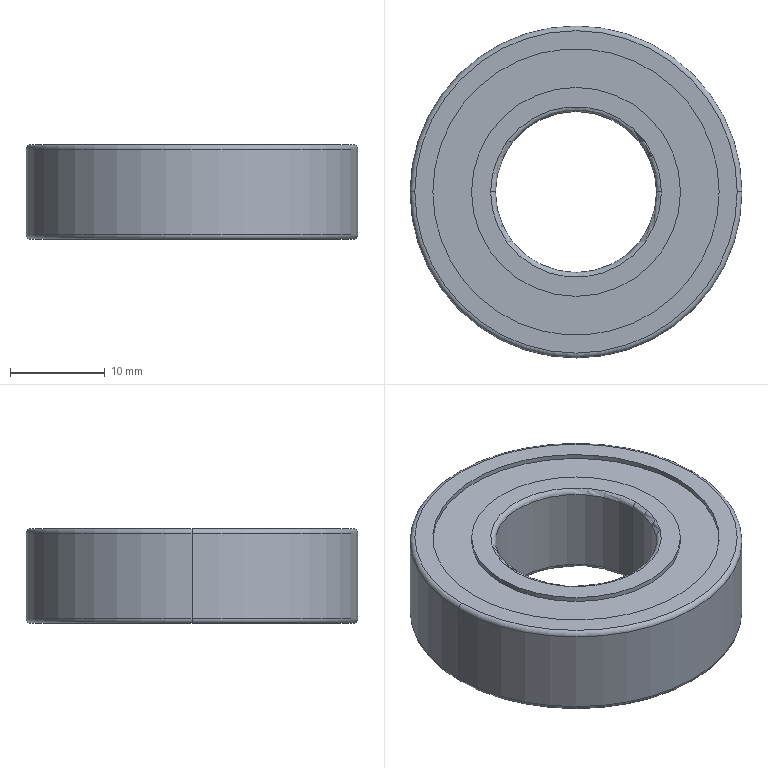Part | NX | features BREP 1 | 1 solid | 26 faces | box 35 x 35 x 10 mm | volume 6999 mm3 | cylinder 12 | torus 8 | plane 6 | commonest cylinder face diameters 22.033 x4 30.197 x4 17 x2 35 x2
STEP:
#1=CARTESIAN_POINT('',(17.5,0.,-4.5));
#2=VERTEX_POINT('',#1);
#3=CARTESIAN_POINT('',(17.5,0.,4.5));
#4=VERTEX_POINT('',#3);
#5=CARTESIAN_POINT('',(17.5,0.,-4.5));
#6=DIRECTION('',(0.,0.,1.));
#7=VECTOR('',#6,1000.);
#8=LINE('',#5,#7);
#9=EDGE_CURVE('',#2,#4,#8,.T.);
#10=ORIENTED_EDGE('',*,*,#9,.F.);
#11=CARTESIAN_POINT('',(-17.5,0.,-4.5));
#12=VERTEX_POINT('',#11);
#13=CARTESIAN_POINT('',(0.,0.,-4.5));
#14=DIRECTION('',(0.,0.,-1.));
#15=DIRECTION('',(-1.,0.,0.));
#16=AXIS2_PLACEMENT_3D('',#13,#14,#15);
#17=CIRCLE('',#16,17.5);
#18=EDGE_CURVE('',#12,#2,#17,.T.);
#19=ORIENTED_EDGE('',*,*,#18,.F.);
#20=CARTESIAN_POINT('',(-17.5,0.,4.5));
#21=VERTEX_POINT('',#20);
#22=CARTESIAN_POINT('',(-17.5,0.,-4.5));
#23=DIRECTION('',(0.,0.,1.));
#24=VECTOR('',#23,1000.);
#25=LINE('',#22,#24);
#26=EDGE_CURVE('',#12,#21,#25,.T.);
#27=ORIENTED_EDGE('',*,*,#26,.T.);
#28=CARTESIAN_POINT('',(0.,0.,4.5));
#29=DIRECTION('',(0.,0.,1.));
#30=DIRECTION('',(1.,0.,0.));
#31=AXIS2_PLACEMENT_3D('',#28,#29,#30);
#32=CIRCLE('',#31,17.5);
#33=EDGE_CURVE('',#4,#21,#32,.T.);
#34=ORIENTED_EDGE('',*,*,#33,.F.);
#35=EDGE_LOOP('',(#10,#19,#27,#34));
#36=FACE_BOUND('',#35,.T.);
#37=CARTESIAN_POINT('',(0.,0.,5.));
#38=DIRECTION('',(0.,0.,-1.));
#39=DIRECTION('',(1.,0.,0.));
#40=AXIS2_PLACEMENT_3D('',#37,#38,#39);
#41=CYLINDRICAL_SURFACE('',#40,17.5);
#42=ADVANCED_FACE('',(#36),#41,.T.);
#43=CARTESIAN_POINT('',(-17.,0.,5.));
#44=VERTEX_POINT('',#43);
#45=CARTESIAN_POINT('',(-17.,0.,4.5));
#46=DIRECTION('',(0.,-1.,0.));
#47=DIRECTION('',(0.,0.,1.));
#48=AXIS2_PLACEMENT_3D('',#45,#46,#47);
#49=CIRCLE('',#48,0.5);
#50=EDGE_CURVE('',#21,#44,#49,.F.);
#51=ORIENTED_EDGE('',*,*,#50,.T.);
#52=CARTESIAN_POINT('',(17.,0.,5.));
#53=VERTEX_POINT('',#52);
#54=CARTESIAN_POINT('',(0.,0.,5.));
#55=DIRECTION('',(0.,0.,1.));
#56=DIRECTION('',(1.,0.,0.));
#57=AXIS2_PLACEMENT_3D('',#54,#55,#56);
#58=CIRCLE('',#57,17.);
#59=EDGE_CURVE('',#53,#44,#58,.T.);
#60=ORIENTED_EDGE('',*,*,#59,.F.);
#61=CARTESIAN_POINT('',(17.,0.,4.5));
#62=DIRECTION('',(0.,1.,0.));
#63=DIRECTION('',(0.,0.,1.));
#64=AXIS2_PLACEMENT_3D('',#61,#62,#63);
#65=CIRCLE('',#64,0.5);
#66=EDGE_CURVE('',#4,#53,#65,.F.);
#67=ORIENTED_EDGE('',*,*,#66,.F.);
#68=ORIENTED_EDGE('',*,*,#33,.T.);
#69=EDGE_LOOP('',(#51,#60,#67,#68));
#70=FACE_BOUND('',#69,.T.);
#71=CARTESIAN_POINT('',(0.,0.,4.5));
#72=DIRECTION('',(0.,0.,1.));
#73=DIRECTION('',(-1.,0.,0.));
#74=AXIS2_PLACEMENT_3D('',#71,#72,#73);
#75=TOROIDAL_SURFACE('',#74,17.,0.5);
#76=ADVANCED_FACE('',(#70),#75,.T.);
#77=CARTESIAN_POINT('',(0.,0.,4.5));
#78=DIRECTION('',(0.,0.,1.));
#79=DIRECTION('',(-1.,0.,0.));
#80=AXIS2_PLACEMENT_3D('',#77,#78,#79);
#81=CIRCLE('',#80,17.5);
#82=EDGE_CURVE('',#21,#4,#81,.T.);
#83=ORIENTED_EDGE('',*,*,#82,.T.);
#84=ORIENTED_EDGE('',*,*,#66,.T.);
#85=CARTESIAN_POINT('',(0.,0.,5.));
#86=DIRECTION('',(0.,0.,1.));
#87=DIRECTION('',(-1.,0.,0.));
#88=AXIS2_PLACEMENT_3D('',#85,#86,#87);
#89=CIRCLE('',#88,17.);
#90=EDGE_CURVE('',#44,#53,#89,.T.);
#91=ORIENTED_EDGE('',*,*,#90,.F.);
#92=ORIENTED_EDGE('',*,*,#50,.F.);
#93=EDGE_LOOP('',(#83,#84,#91,#92));
#94=FACE_BOUND('',#93,.T.);
#95=CARTESIAN_POINT('',(0.,0.,4.5));
#96=DIRECTION('',(0.,0.,1.));
#97=DIRECTION('',(-1.,0.,0.));
#98=AXIS2_PLACEMENT_3D('',#95,#96,#97);
#99=TOROIDAL_SURFACE('',#98,17.,0.5);
#100=ADVANCED_FACE('',(#94),#99,.T.);
#101=ORIENTED_EDGE('',*,*,#90,.T.);
#102=ORIENTED_EDGE('',*,*,#59,.T.);
#103=EDGE_LOOP('',(#101,#102));
#104=FACE_BOUND('',#103,.T.);
#105=CARTESIAN_POINT('',(15.098,0.,5.));
#106=VERTEX_POINT('',#105);
#107=CARTESIAN_POINT('',(-15.098,0.,5.));
#108=VERTEX_POINT('',#107);
#109=CARTESIAN_POINT('',(0.,0.,5.));
#110=DIRECTION('',(0.,0.,-1.));
#111=DIRECTION('',(1.,0.,0.));
#112=AXIS2_PLACEMENT_3D('',#109,#110,#111);
#113=CIRCLE('',#112,15.098);
#114=EDGE_CURVE('',#106,#108,#113,.T.);
#115=ORIENTED_EDGE('',*,*,#114,.T.);
#116=CARTESIAN_POINT('',(0.,0.,5.));
#117=DIRECTION('',(0.,0.,-1.));
#118=DIRECTION('',(-1.,0.,0.));
#119=AXIS2_PLACEMENT_3D('',#116,#117,#118);
#120=CIRCLE('',#119,15.098);
#121=EDGE_CURVE('',#108,#106,#120,.T.);
#122=ORIENTED_EDGE('',*,*,#121,.T.);
#123=EDGE_LOOP('',(#115,#122));
#124=FACE_BOUND('',#123,.T.);
#125=CARTESIAN_POINT('',(0.,0.,5.));
#126=DIRECTION('',(0.,0.,1.));
#127=DIRECTION('',(-1.,0.,0.));
#128=AXIS2_PLACEMENT_3D('',#125,#126,#127);
#129=PLANE('',#128);
#130=ADVANCED_FACE('',(#104,#124),#129,.T.);
#131=CARTESIAN_POINT('',(15.098,0.,4.5));
#132=VERTEX_POINT('',#131);
#133=CARTESIAN_POINT('',(-15.098,0.,4.5));
#134=VERTEX_POINT('',#133);
#135=CARTESIAN_POINT('',(0.,0.,4.5));
#136=DIRECTION('',(0.,0.,1.));
#137=DIRECTION('',(1.,0.,0.));
#138=AXIS2_PLACEMENT_3D('',#135,#136,#137);
#139=CIRCLE('',#138,15.098);
#140=EDGE_CURVE('',#132,#134,#139,.T.);
#141=ORIENTED_EDGE('',*,*,#140,.F.);
#142=CARTESIAN_POINT('',(15.098,0.,5.));
#143=DIRECTION('',(0.,0.,-1.));
#144=VECTOR('',#143,1000.);
#145=LINE('',#142,#144);
#146=EDGE_CURVE('',#106,#132,#145,.T.);
#147=ORIENTED_EDGE('',*,*,#146,.F.);
#148=ORIENTED_EDGE('',*,*,#121,.F.);
#149=CARTESIAN_POINT('',(-15.098,0.,5.));
#150=DIRECTION('',(0.,0.,-1.));
#151=VECTOR('',#150,1000.);
#152=LINE('',#149,#151);
#153=EDGE_CURVE('',#108,#134,#152,.T.);
#154=ORIENTED_EDGE('',*,*,#153,.T.);
#155=EDGE_LOOP('',(#141,#147,#148,#154));
#156=FACE_BOUND('',#155,.T.);
#157=CARTESIAN_POINT('',(0.,0.,4.5));
#158=DIRECTION('',(0.,0.,1.));
#159=DIRECTION('',(-1.,0.,0.));
#160=AXIS2_PLACEMENT_3D('',#157,#158,#159);
#161=CYLINDRICAL_SURFACE('',#160,15.098);
#162=ADVANCED_FACE('',(#156),#161,.F.);
#163=ORIENTED_EDGE('',*,*,#153,.F.);
#164=ORIENTED_EDGE('',*,*,#114,.F.);
#165=ORIENTED_EDGE('',*,*,#146,.T.);
#166=CARTESIAN_POINT('',(0.,0.,4.5));
#167=DIRECTION('',(0.,0.,1.));
#168=DIRECTION('',(-1.,0.,0.));
#169=AXIS2_PLACEMENT_3D('',#166,#167,#168);
#170=CIRCLE('',#169,15.098);
#171=EDGE_CURVE('',#134,#132,#170,.T.);
#172=ORIENTED_EDGE('',*,*,#171,.F.);
#173=EDGE_LOOP('',(#163,#164,#165,#172));
#174=FACE_BOUND('',#173,.T.);
#175=CARTESIAN_POINT('',(0.,0.,4.5));
#176=DIRECTION('',(0.,0.,1.));
#177=DIRECTION('',(-1.,0.,0.));
#178=AXIS2_PLACEMENT_3D('',#175,#176,#177);
#179=CYLINDRICAL_SURFACE('',#178,15.098);
#180=ADVANCED_FACE('',(#174),#179,.F.);
#181=ORIENTED_EDGE('',*,*,#171,.T.);
#182=ORIENTED_EDGE('',*,*,#140,.T.);
#183=EDGE_LOOP('',(#181,#182));
#184=FACE_BOUND('',#183,.T.);
#185=CARTESIAN_POINT('',(11.017,0.,4.5));
#186=VERTEX_POINT('',#185);
#187=CARTESIAN_POINT('',(-11.017,0.,4.5));
#188=VERTEX_POINT('',#187);
#189=CARTESIAN_POINT('',(0.,0.,4.5));
#190=DIRECTION('',(0.,0.,-1.));
#191=DIRECTION('',(1.,0.,0.));
#192=AXIS2_PLACEMENT_3D('',#189,#190,#191);
#193=CIRCLE('',#192,11.017);
#194=EDGE_CURVE('',#186,#188,#193,.T.);
#195=ORIENTED_EDGE('',*,*,#194,.T.);
#196=CARTESIAN_POINT('',(0.,0.,4.5));
#197=DIRECTION('',(0.,0.,-1.));
#198=DIRECTION('',(-1.,0.,0.));
#199=AXIS2_PLACEMENT_3D('',#196,#197,#198);
#200=CIRCLE('',#199,11.017);
#201=EDGE_CURVE('',#188,#186,#200,.T.);
#202=ORIENTED_EDGE('',*,*,#201,.T.);
#203=EDGE_LOOP('',(#195,#202));
#204=FACE_BOUND('',#203,.T.);
#205=CARTESIAN_POINT('',(0.,0.,4.5));
#206=DIRECTION('',(0.,0.,1.));
#207=DIRECTION('',(-1.,0.,0.));
#208=AXIS2_PLACEMENT_3D('',#205,#206,#207);
#209=PLANE('',#208);
#210=ADVANCED_FACE('',(#184,#204),#209,.T.);
#211=CARTESIAN_POINT('',(-11.017,0.,5.));
#212=VERTEX_POINT('',#211);
#213=CARTESIAN_POINT('',(-11.017,0.,5.));
#214=DIRECTION('',(0.,0.,-1.));
#215=VECTOR('',#214,1000.);
#216=LINE('',#213,#215);
#217=EDGE_CURVE('',#188,#212,#216,.F.);
#218=ORIENTED_EDGE('',*,*,#217,.T.);
#219=CARTESIAN_POINT('',(11.017,0.,5.));
#220=VERTEX_POINT('',#219);
#221=CARTESIAN_POINT('',(0.,0.,5.));
#222=DIRECTION('',(0.,0.,1.));
#223=DIRECTION('',(1.,0.,0.));
#224=AXIS2_PLACEMENT_3D('',#221,#222,#223);
#225=CIRCLE('',#224,11.017);
#226=EDGE_CURVE('',#220,#212,#225,.T.);
#227=ORIENTED_EDGE('',*,*,#226,.F.);
#228=CARTESIAN_POINT('',(11.017,0.,5.));
#229=DIRECTION('',(0.,0.,-1.));
#230=VECTOR('',#229,1000.);
#231=LINE('',#228,#230);
#232=EDGE_CURVE('',#186,#220,#231,.F.);
#233=ORIENTED_EDGE('',*,*,#232,.F.);
#234=ORIENTED_EDGE('',*,*,#201,.F.);
#235=EDGE_LOOP('',(#218,#227,#233,#234));
#236=FACE_BOUND('',#235,.T.);
#237=CARTESIAN_POINT('',(0.,0.,4.5));
#238=DIRECTION('',(0.,0.,1.));
#239=DIRECTION('',(-1.,0.,0.));
#240=AXIS2_PLACEMENT_3D('',#237,#238,#239);
#241=CYLINDRICAL_SURFACE('',#240,11.017);
#242=ADVANCED_FACE('',(#236),#241,.T.);
#243=ORIENTED_EDGE('',*,*,#194,.F.);
#244=ORIENTED_EDGE('',*,*,#232,.T.);
#245=CARTESIAN_POINT('',(0.,0.,5.));
#246=DIRECTION('',(0.,0.,1.));
#247=DIRECTION('',(-1.,0.,0.));
#248=AXIS2_PLACEMENT_3D('',#245,#246,#247);
#249=CIRCLE('',#248,11.017);
#250=EDGE_CURVE('',#212,#220,#249,.T.);
#251=ORIENTED_EDGE('',*,*,#250,.F.);
#252=ORIENTED_EDGE('',*,*,#217,.F.);
#253=EDGE_LOOP('',(#243,#244,#251,#252));
#254=FACE_BOUND('',#253,.T.);
#255=CARTESIAN_POINT('',(0.,0.,4.5));
#256=DIRECTION('',(0.,0.,1.));
#257=DIRECTION('',(-1.,0.,0.));
#258=AXIS2_PLACEMENT_3D('',#255,#256,#257);
#259=CYLINDRICAL_SURFACE('',#258,11.017);
#260=ADVANCED_FACE('',(#254),#259,.T.);
#261=ORIENTED_EDGE('',*,*,#250,.T.);
#262=ORIENTED_EDGE('',*,*,#226,.T.);
#263=EDGE_LOOP('',(#261,#262));
#264=FACE_BOUND('',#263,.T.);
#265=CARTESIAN_POINT('',(-9.,0.,5.));
#266=VERTEX_POINT('',#265);
#267=CARTESIAN_POINT('',(9.,0.,5.));
#268=VERTEX_POINT('',#267);
#269=CARTESIAN_POINT('',(0.,0.,5.));
#270=DIRECTION('',(0.,0.,-1.));
#271=DIRECTION('',(-1.,0.,0.));
#272=AXIS2_PLACEMENT_3D('',#269,#270,#271);
#273=CIRCLE('',#272,9.);
#274=EDGE_CURVE('',#266,#268,#273,.T.);
#275=ORIENTED_EDGE('',*,*,#274,.T.);
#276=CARTESIAN_POINT('',(0.,0.,5.));
#277=DIRECTION('',(0.,0.,-1.));
#278=DIRECTION('',(1.,0.,0.));
#279=AXIS2_PLACEMENT_3D('',#276,#277,#278);
#280=CIRCLE('',#279,9.);
#281=EDGE_CURVE('',#268,#266,#280,.T.);
#282=ORIENTED_EDGE('',*,*,#281,.T.);
#283=EDGE_LOOP('',(#275,#282));
#284=FACE_BOUND('',#283,.T.);
#285=CARTESIAN_POINT('',(0.,0.,5.));
#286=DIRECTION('',(0.,0.,1.));
#287=DIRECTION('',(-1.,0.,0.));
#288=AXIS2_PLACEMENT_3D('',#285,#286,#287);
#289=PLANE('',#288);
#290=ADVANCED_FACE('',(#264,#284),#289,.T.);
#291=ORIENTED_EDGE('',*,*,#281,.F.);
#292=CARTESIAN_POINT('',(8.5,0.,4.5));
#293=VERTEX_POINT('',#292);
#294=CARTESIAN_POINT('',(9.,0.,4.5));
#295=DIRECTION('',(0.,1.,0.));
#296=DIRECTION('',(-1.,0.,0.));
#297=AXIS2_PLACEMENT_3D('',#294,#295,#296);
#298=CIRCLE('',#297,0.5);
#299=EDGE_CURVE('',#293,#268,#298,.T.);
#300=ORIENTED_EDGE('',*,*,#299,.F.);
#301=CARTESIAN_POINT('',(-8.5,0.,4.5));
#302=VERTEX_POINT('',#301);
#303=CARTESIAN_POINT('',(0.,0.,4.5));
#304=DIRECTION('',(0.,0.,-1.));
#305=DIRECTION('',(1.,0.,0.));
#306=AXIS2_PLACEMENT_3D('',#303,#304,#305);
#307=CIRCLE('',#306,8.5);
#308=EDGE_CURVE('',#293,#302,#307,.T.);
#309=ORIENTED_EDGE('',*,*,#308,.T.);
#310=CARTESIAN_POINT('',(-9.,0.,4.5));
#311=DIRECTION('',(0.,-1.,0.));
#312=DIRECTION('',(1.,0.,0.));
#313=AXIS2_PLACEMENT_3D('',#310,#311,#312);
#314=CIRCLE('',#313,0.5);
#315=EDGE_CURVE('',#302,#266,#314,.T.);
#316=ORIENTED_EDGE('',*,*,#315,.T.);
#317=EDGE_LOOP('',(#291,#300,#309,#316));
#318=FACE_BOUND('',#317,.T.);
#319=CARTESIAN_POINT('',(0.,0.,4.5));
#320=DIRECTION('',(0.,0.,1.));
#321=DIRECTION('',(-1.,0.,0.));
#322=AXIS2_PLACEMENT_3D('',#319,#320,#321);
#323=TOROIDAL_SURFACE('',#322,9.,0.5);
#324=ADVANCED_FACE('',(#318),#323,.T.);
#325=ORIENTED_EDGE('',*,*,#315,.F.);
#326=CARTESIAN_POINT('',(0.,0.,4.5));
#327=DIRECTION('',(0.,0.,-1.));
#328=DIRECTION('',(-1.,0.,0.));
#329=AXIS2_PLACEMENT_3D('',#326,#327,#328);
#330=CIRCLE('',#329,8.5);
#331=EDGE_CURVE('',#302,#293,#330,.T.);
#332=ORIENTED_EDGE('',*,*,#331,.T.);
#333=ORIENTED_EDGE('',*,*,#299,.T.);
#334=ORIENTED_EDGE('',*,*,#274,.F.);
#335=EDGE_LOOP('',(#325,#332,#333,#334));
#336=FACE_BOUND('',#335,.T.);
#337=CARTESIAN_POINT('',(0.,0.,4.5));
#338=DIRECTION('',(0.,0.,1.));
#339=DIRECTION('',(-1.,0.,0.));
#340=AXIS2_PLACEMENT_3D('',#337,#338,#339);
#341=TOROIDAL_SURFACE('',#340,9.,0.5);
#342=ADVANCED_FACE('',(#336),#341,.T.);
#343=ORIENTED_EDGE('',*,*,#331,.F.);
#344=CARTESIAN_POINT('',(-8.5,0.,-4.5));
#345=VERTEX_POINT('',#344);
#346=CARTESIAN_POINT('',(-8.5,0.,-4.5));
#347=DIRECTION('',(0.,0.,1.));
#348=VECTOR('',#347,1000.);
#349=LINE('',#346,#348);
#350=EDGE_CURVE('',#302,#345,#349,.F.);
#351=ORIENTED_EDGE('',*,*,#350,.T.);
#352=CARTESIAN_POINT('',(8.5,0.,-4.5));
#353=VERTEX_POINT('',#352);
#354=CARTESIAN_POINT('',(0.,0.,-4.5));
#355=DIRECTION('',(0.,0.,1.));
#356=DIRECTION('',(1.,0.,0.));
#357=AXIS2_PLACEMENT_3D('',#354,#355,#356);
#358=CIRCLE('',#357,8.5);
#359=EDGE_CURVE('',#353,#345,#358,.T.);
#360=ORIENTED_EDGE('',*,*,#359,.F.);
#361=CARTESIAN_POINT('',(8.5,0.,-4.5));
#362=DIRECTION('',(0.,0.,1.));
#363=VECTOR('',#362,1000.);
#364=LINE('',#361,#363);
#365=EDGE_CURVE('',#293,#353,#364,.F.);
#366=ORIENTED_EDGE('',*,*,#365,.F.);
#367=EDGE_LOOP('',(#343,#351,#360,#366));
#368=FACE_BOUND('',#367,.T.);
#369=CARTESIAN_POINT('',(0.,0.,5.));
#370=DIRECTION('',(0.,0.,-1.));
#371=DIRECTION('',(1.,0.,0.));
#372=AXIS2_PLACEMENT_3D('',#369,#370,#371);
#373=CYLINDRICAL_SURFACE('',#372,8.5);
#374=ADVANCED_FACE('',(#368),#373,.F.);
#375=ORIENTED_EDGE('',*,*,#365,.T.);
#376=CARTESIAN_POINT('',(0.,0.,-4.5));
#377=DIRECTION('',(0.,0.,1.));
#378=DIRECTION('',(-1.,0.,0.));
#379=AXIS2_PLACEMENT_3D('',#376,#377,#378);
#380=CIRCLE('',#379,8.5);
#381=EDGE_CURVE('',#345,#353,#380,.T.);
#382=ORIENTED_EDGE('',*,*,#381,.F.);
#383=ORIENTED_EDGE('',*,*,#350,.F.);
#384=ORIENTED_EDGE('',*,*,#308,.F.);
#385=EDGE_LOOP('',(#375,#382,#383,#384));
#386=FACE_BOUND('',#385,.T.);
#387=CARTESIAN_POINT('',(0.,0.,5.));
#388=DIRECTION('',(0.,0.,-1.));
#389=DIRECTION('',(1.,0.,0.));
#390=AXIS2_PLACEMENT_3D('',#387,#388,#389);
#391=CYLINDRICAL_SURFACE('',#390,8.5);
#392=ADVANCED_FACE('',(#386),#391,.F.);
#393=ORIENTED_EDGE('',*,*,#381,.T.);
#394=CARTESIAN_POINT('',(9.,0.,-5.));
#395=VERTEX_POINT('',#394);
#396=CARTESIAN_POINT('',(9.,0.,-4.5));
#397=DIRECTION('',(0.,1.,0.));
#398=DIRECTION('',(0.,0.,-1.));
#399=AXIS2_PLACEMENT_3D('',#396,#397,#398);
#400=CIRCLE('',#399,0.5);
#401=EDGE_CURVE('',#395,#353,#400,.T.);
#402=ORIENTED_EDGE('',*,*,#401,.F.);
#403=CARTESIAN_POINT('',(-9.,0.,-5.));
#404=VERTEX_POINT('',#403);
#405=CARTESIAN_POINT('',(0.,0.,-5.));
#406=DIRECTION('',(0.,0.,1.));
#407=DIRECTION('',(-1.,0.,0.));
#408=AXIS2_PLACEMENT_3D('',#405,#406,#407);
#409=CIRCLE('',#408,9.);
#410=EDGE_CURVE('',#404,#395,#409,.T.);
#411=ORIENTED_EDGE('',*,*,#410,.F.);
#412=CARTESIAN_POINT('',(-9.,0.,-4.5));
#413=DIRECTION('',(0.,-1.,0.));
#414=DIRECTION('',(0.,0.,-1.));
#415=AXIS2_PLACEMENT_3D('',#412,#413,#414);
#416=CIRCLE('',#415,0.5);
#417=EDGE_CURVE('',#404,#345,#416,.T.);
#418=ORIENTED_EDGE('',*,*,#417,.T.);
#419=EDGE_LOOP('',(#393,#402,#411,#418));
#420=FACE_BOUND('',#419,.T.);
#421=CARTESIAN_POINT('',(0.,0.,-4.5));
#422=DIRECTION('',(0.,0.,1.));
#423=DIRECTION('',(-1.,0.,0.));
#424=AXIS2_PLACEMENT_3D('',#421,#422,#423);
#425=TOROIDAL_SURFACE('',#424,9.,0.5);
#426=ADVANCED_FACE('',(#420),#425,.T.);
#427=ORIENTED_EDGE('',*,*,#417,.F.);
#428=CARTESIAN_POINT('',(0.,0.,-5.));
#429=DIRECTION('',(0.,0.,1.));
#430=DIRECTION('',(1.,0.,0.));
#431=AXIS2_PLACEMENT_3D('',#428,#429,#430);
#432=CIRCLE('',#431,9.);
#433=EDGE_CURVE('',#395,#404,#432,.T.);
#434=ORIENTED_EDGE('',*,*,#433,.F.);
#435=ORIENTED_EDGE('',*,*,#401,.T.);
#436=ORIENTED_EDGE('',*,*,#359,.T.);
#437=EDGE_LOOP('',(#427,#434,#435,#436));
#438=FACE_BOUND('',#437,.T.);
#439=CARTESIAN_POINT('',(0.,0.,-4.5));
#440=DIRECTION('',(0.,0.,1.));
#441=DIRECTION('',(-1.,0.,0.));
#442=AXIS2_PLACEMENT_3D('',#439,#440,#441);
#443=TOROIDAL_SURFACE('',#442,9.,0.5);
#444=ADVANCED_FACE('',(#438),#443,.T.);
#445=CARTESIAN_POINT('',(-11.017,0.,-5.));
#446=VERTEX_POINT('',#445);
#447=CARTESIAN_POINT('',(11.017,0.,-5.));
#448=VERTEX_POINT('',#447);
#449=CARTESIAN_POINT('',(0.,0.,-5.));
#450=DIRECTION('',(0.,0.,-1.));
#451=DIRECTION('',(-1.,0.,0.));
#452=AXIS2_PLACEMENT_3D('',#449,#450,#451);
#453=CIRCLE('',#452,11.017);
#454=EDGE_CURVE('',#446,#448,#453,.T.);
#455=ORIENTED_EDGE('',*,*,#454,.T.);
#456=CARTESIAN_POINT('',(0.,0.,-5.));
#457=DIRECTION('',(0.,0.,-1.));
#458=DIRECTION('',(1.,0.,0.));
#459=AXIS2_PLACEMENT_3D('',#456,#457,#458);
#460=CIRCLE('',#459,11.017);
#461=EDGE_CURVE('',#448,#446,#460,.T.);
#462=ORIENTED_EDGE('',*,*,#461,.T.);
#463=EDGE_LOOP('',(#455,#462));
#464=FACE_BOUND('',#463,.T.);
#465=ORIENTED_EDGE('',*,*,#410,.T.);
#466=ORIENTED_EDGE('',*,*,#433,.T.);
#467=EDGE_LOOP('',(#465,#466));
#468=FACE_BOUND('',#467,.T.);
#469=CARTESIAN_POINT('',(0.,0.,-5.));
#470=DIRECTION('',(0.,0.,1.));
#471=DIRECTION('',(-1.,0.,0.));
#472=AXIS2_PLACEMENT_3D('',#469,#470,#471);
#473=PLANE('',#472);
#474=ADVANCED_FACE('',(#464,#468),#473,.F.);
#475=CARTESIAN_POINT('',(-11.017,0.,-4.5));
#476=VERTEX_POINT('',#475);
#477=CARTESIAN_POINT('',(11.017,0.,-4.5));
#478=VERTEX_POINT('',#477);
#479=CARTESIAN_POINT('',(0.,0.,-4.5));
#480=DIRECTION('',(0.,0.,1.));
#481=DIRECTION('',(-1.,0.,0.));
#482=AXIS2_PLACEMENT_3D('',#479,#480,#481);
#483=CIRCLE('',#482,11.017);
#484=EDGE_CURVE('',#476,#478,#483,.T.);
#485=ORIENTED_EDGE('',*,*,#484,.F.);
#486=CARTESIAN_POINT('',(-11.017,0.,-5.));
#487=DIRECTION('',(0.,0.,1.));
#488=VECTOR('',#487,1000.);
#489=LINE('',#486,#488);
#490=EDGE_CURVE('',#476,#446,#489,.F.);
#491=ORIENTED_EDGE('',*,*,#490,.T.);
#492=ORIENTED_EDGE('',*,*,#461,.F.);
#493=CARTESIAN_POINT('',(11.017,0.,-5.));
#494=DIRECTION('',(0.,0.,1.));
#495=VECTOR('',#494,1000.);
#496=LINE('',#493,#495);
#497=EDGE_CURVE('',#478,#448,#496,.F.);
#498=ORIENTED_EDGE('',*,*,#497,.F.);
#499=EDGE_LOOP('',(#485,#491,#492,#498));
#500=FACE_BOUND('',#499,.T.);
#501=CARTESIAN_POINT('',(0.,0.,-4.5));
#502=DIRECTION('',(0.,0.,-1.));
#503=DIRECTION('',(1.,0.,0.));
#504=AXIS2_PLACEMENT_3D('',#501,#502,#503);
#505=CYLINDRICAL_SURFACE('',#504,11.017);
#506=ADVANCED_FACE('',(#500),#505,.T.);
#507=ORIENTED_EDGE('',*,*,#497,.T.);
#508=ORIENTED_EDGE('',*,*,#454,.F.);
#509=ORIENTED_EDGE('',*,*,#490,.F.);
#510=CARTESIAN_POINT('',(0.,0.,-4.5));
#511=DIRECTION('',(0.,0.,1.));
#512=DIRECTION('',(1.,0.,0.));
#513=AXIS2_PLACEMENT_3D('',#510,#511,#512);
#514=CIRCLE('',#513,11.017);
#515=EDGE_CURVE('',#478,#476,#514,.T.);
#516=ORIENTED_EDGE('',*,*,#515,.F.);
#517=EDGE_LOOP('',(#507,#508,#509,#516));
#518=FACE_BOUND('',#517,.T.);
#519=CARTESIAN_POINT('',(0.,0.,-4.5));
#520=DIRECTION('',(0.,0.,-1.));
#521=DIRECTION('',(1.,0.,0.));
#522=AXIS2_PLACEMENT_3D('',#519,#520,#521);
#523=CYLINDRICAL_SURFACE('',#522,11.017);
#524=ADVANCED_FACE('',(#518),#523,.T.);
#525=CARTESIAN_POINT('',(-15.098,0.,-4.5));
#526=VERTEX_POINT('',#525);
#527=CARTESIAN_POINT('',(15.098,0.,-4.5));
#528=VERTEX_POINT('',#527);
#529=CARTESIAN_POINT('',(0.,0.,-4.5));
#530=DIRECTION('',(0.,0.,-1.));
#531=DIRECTION('',(-1.,0.,0.));
#532=AXIS2_PLACEMENT_3D('',#529,#530,#531);
#533=CIRCLE('',#532,15.098);
#534=EDGE_CURVE('',#526,#528,#533,.T.);
#535=ORIENTED_EDGE('',*,*,#534,.T.);
#536=CARTESIAN_POINT('',(0.,0.,-4.5));
#537=DIRECTION('',(0.,0.,-1.));
#538=DIRECTION('',(1.,0.,0.));
#539=AXIS2_PLACEMENT_3D('',#536,#537,#538);
#540=CIRCLE('',#539,15.098);
#541=EDGE_CURVE('',#528,#526,#540,.T.);
#542=ORIENTED_EDGE('',*,*,#541,.T.);
#543=EDGE_LOOP('',(#535,#542));
#544=FACE_BOUND('',#543,.T.);
#545=ORIENTED_EDGE('',*,*,#515,.T.);
#546=ORIENTED_EDGE('',*,*,#484,.T.);
#547=EDGE_LOOP('',(#545,#546));
#548=FACE_BOUND('',#547,.T.);
#549=CARTESIAN_POINT('',(0.,0.,-4.5));
#550=DIRECTION('',(0.,0.,-1.));
#551=DIRECTION('',(-1.,0.,0.));
#552=AXIS2_PLACEMENT_3D('',#549,#550,#551);
#553=PLANE('',#552);
#554=ADVANCED_FACE('',(#544,#548),#553,.T.);
#555=CARTESIAN_POINT('',(15.098,0.,-5.));
#556=VERTEX_POINT('',#555);
#557=CARTESIAN_POINT('',(15.098,0.,-5.));
#558=DIRECTION('',(0.,0.,1.));
#559=VECTOR('',#558,1000.);
#560=LINE('',#557,#559);
#561=EDGE_CURVE('',#556,#528,#560,.T.);
#562=ORIENTED_EDGE('',*,*,#561,.F.);
#563=CARTESIAN_POINT('',(-15.098,0.,-5.));
#564=VERTEX_POINT('',#563);
#565=CARTESIAN_POINT('',(0.,0.,-5.));
#566=DIRECTION('',(0.,0.,1.));
#567=DIRECTION('',(-1.,0.,0.));
#568=AXIS2_PLACEMENT_3D('',#565,#566,#567);
#569=CIRCLE('',#568,15.098);
#570=EDGE_CURVE('',#564,#556,#569,.T.);
#571=ORIENTED_EDGE('',*,*,#570,.F.);
#572=CARTESIAN_POINT('',(-15.098,0.,-5.));
#573=DIRECTION('',(0.,0.,1.));
#574=VECTOR('',#573,1000.);
#575=LINE('',#572,#574);
#576=EDGE_CURVE('',#564,#526,#575,.T.);
#577=ORIENTED_EDGE('',*,*,#576,.T.);
#578=ORIENTED_EDGE('',*,*,#541,.F.);
#579=EDGE_LOOP('',(#562,#571,#577,#578));
#580=FACE_BOUND('',#579,.T.);
#581=CARTESIAN_POINT('',(0.,0.,-4.5));
#582=DIRECTION('',(0.,0.,-1.));
#583=DIRECTION('',(1.,0.,0.));
#584=AXIS2_PLACEMENT_3D('',#581,#582,#583);
#585=CYLINDRICAL_SURFACE('',#584,15.098);
#586=ADVANCED_FACE('',(#580),#585,.F.);
#587=ORIENTED_EDGE('',*,*,#534,.F.);
#588=ORIENTED_EDGE('',*,*,#576,.F.);
#589=CARTESIAN_POINT('',(0.,0.,-5.));
#590=DIRECTION('',(0.,0.,1.));
#591=DIRECTION('',(1.,0.,0.));
#592=AXIS2_PLACEMENT_3D('',#589,#590,#591);
#593=CIRCLE('',#592,15.098);
#594=EDGE_CURVE('',#556,#564,#593,.T.);
#595=ORIENTED_EDGE('',*,*,#594,.F.);
#596=ORIENTED_EDGE('',*,*,#561,.T.);
#597=EDGE_LOOP('',(#587,#588,#595,#596));
#598=FACE_BOUND('',#597,.T.);
#599=CARTESIAN_POINT('',(0.,0.,-4.5));
#600=DIRECTION('',(0.,0.,-1.));
#601=DIRECTION('',(1.,0.,0.));
#602=AXIS2_PLACEMENT_3D('',#599,#600,#601);
#603=CYLINDRICAL_SURFACE('',#602,15.098);
#604=ADVANCED_FACE('',(#598),#603,.F.);
#605=CARTESIAN_POINT('',(-17.,0.,-5.));
#606=VERTEX_POINT('',#605);
#607=CARTESIAN_POINT('',(17.,0.,-5.));
#608=VERTEX_POINT('',#607);
#609=CARTESIAN_POINT('',(0.,0.,-5.));
#610=DIRECTION('',(0.,0.,-1.));
#611=DIRECTION('',(-1.,0.,0.));
#612=AXIS2_PLACEMENT_3D('',#609,#610,#611);
#613=CIRCLE('',#612,17.);
#614=EDGE_CURVE('',#606,#608,#613,.T.);
#615=ORIENTED_EDGE('',*,*,#614,.T.);
#616=CARTESIAN_POINT('',(0.,0.,-5.));
#617=DIRECTION('',(0.,0.,-1.));
#618=DIRECTION('',(1.,0.,0.));
#619=AXIS2_PLACEMENT_3D('',#616,#617,#618);
#620=CIRCLE('',#619,17.);
#621=EDGE_CURVE('',#608,#606,#620,.T.);
#622=ORIENTED_EDGE('',*,*,#621,.T.);
#623=EDGE_LOOP('',(#615,#622));
#624=FACE_BOUND('',#623,.T.);
#625=ORIENTED_EDGE('',*,*,#594,.T.);
#626=ORIENTED_EDGE('',*,*,#570,.T.);
#627=EDGE_LOOP('',(#625,#626));
#628=FACE_BOUND('',#627,.T.);
#629=CARTESIAN_POINT('',(0.,0.,-5.));
#630=DIRECTION('',(0.,0.,1.));
#631=DIRECTION('',(-1.,0.,0.));
#632=AXIS2_PLACEMENT_3D('',#629,#630,#631);
#633=PLANE('',#632);
#634=ADVANCED_FACE('',(#624,#628),#633,.F.);
#635=ORIENTED_EDGE('',*,*,#621,.F.);
#636=CARTESIAN_POINT('',(17.,0.,-4.5));
#637=DIRECTION('',(0.,1.,0.));
#638=DIRECTION('',(1.,0.,0.));
#639=AXIS2_PLACEMENT_3D('',#636,#637,#638);
#640=CIRCLE('',#639,0.5);
#641=EDGE_CURVE('',#2,#608,#640,.T.);
#642=ORIENTED_EDGE('',*,*,#641,.F.);
#643=CARTESIAN_POINT('',(0.,0.,-4.5));
#644=DIRECTION('',(0.,0.,-1.));
#645=DIRECTION('',(1.,0.,0.));
#646=AXIS2_PLACEMENT_3D('',#643,#644,#645);
#647=CIRCLE('',#646,17.5);
#648=EDGE_CURVE('',#2,#12,#647,.T.);
#649=ORIENTED_EDGE('',*,*,#648,.T.);
#650=CARTESIAN_POINT('',(-17.,0.,-4.5));
#651=DIRECTION('',(0.,-1.,0.));
#652=DIRECTION('',(-1.,0.,0.));
#653=AXIS2_PLACEMENT_3D('',#650,#651,#652);
#654=CIRCLE('',#653,0.5);
#655=EDGE_CURVE('',#12,#606,#654,.T.);
#656=ORIENTED_EDGE('',*,*,#655,.T.);
#657=EDGE_LOOP('',(#635,#642,#649,#656));
#658=FACE_BOUND('',#657,.T.);
#659=CARTESIAN_POINT('',(0.,0.,-4.5));
#660=DIRECTION('',(0.,0.,1.));
#661=DIRECTION('',(-1.,0.,0.));
#662=AXIS2_PLACEMENT_3D('',#659,#660,#661);
#663=TOROIDAL_SURFACE('',#662,17.,0.5);
#664=ADVANCED_FACE('',(#658),#663,.T.);
#665=ORIENTED_EDGE('',*,*,#655,.F.);
#666=ORIENTED_EDGE('',*,*,#18,.T.);
#667=ORIENTED_EDGE('',*,*,#641,.T.);
#668=ORIENTED_EDGE('',*,*,#614,.F.);
#669=EDGE_LOOP('',(#665,#666,#667,#668));
#670=FACE_BOUND('',#669,.T.);
#671=CARTESIAN_POINT('',(0.,0.,-4.5));
#672=DIRECTION('',(0.,0.,1.));
#673=DIRECTION('',(-1.,0.,0.));
#674=AXIS2_PLACEMENT_3D('',#671,#672,#673);
#675=TOROIDAL_SURFACE('',#674,17.,0.5);
#676=ADVANCED_FACE('',(#670),#675,.T.);
#677=ORIENTED_EDGE('',*,*,#82,.F.);
#678=ORIENTED_EDGE('',*,*,#26,.F.);
#679=ORIENTED_EDGE('',*,*,#648,.F.);
#680=ORIENTED_EDGE('',*,*,#9,.T.);
#681=EDGE_LOOP('',(#677,#678,#679,#680));
#682=FACE_BOUND('',#681,.T.);
#683=CARTESIAN_POINT('',(0.,0.,5.));
#684=DIRECTION('',(0.,0.,-1.));
#685=DIRECTION('',(1.,0.,0.));
#686=AXIS2_PLACEMENT_3D('',#683,#684,#685);
#687=CYLINDRICAL_SURFACE('',#686,17.5);
#688=ADVANCED_FACE('',(#682),#687,.T.);
#689=CLOSED_SHELL('',(#42,#76,#100,#130,#162,#180,#210,#242,#260,#290,#324,#342,#374,#392,#426,#444,#474,#506,#524,#554,#586,#604,#634,#664,#676,#688));
#690=MANIFOLD_SOLID_BREP('',#689);
#691=(LENGTH_UNIT()NAMED_UNIT(*)SI_UNIT(.MILLI.,.METRE.));
#692=UNCERTAINTY_MEASURE_WITH_UNIT(LENGTH_MEASURE(0.00001),#691,'','');
#693=(NAMED_UNIT(*)PLANE_ANGLE_UNIT()SI_UNIT($,.RADIAN.));
#694=(NAMED_UNIT(*)SI_UNIT($,.STERADIAN.)SOLID_ANGLE_UNIT());
#695=(GEOMETRIC_REPRESENTATION_CONTEXT(3)GLOBAL_UNCERTAINTY_ASSIGNED_CONTEXT((#692))GLOBAL_UNIT_ASSIGNED_CONTEXT((#691,#693,#694))REPRESENTATION_CONTEXT('',''));
#696=ADVANCED_BREP_SHAPE_REPRESENTATION('',(#690),#695);